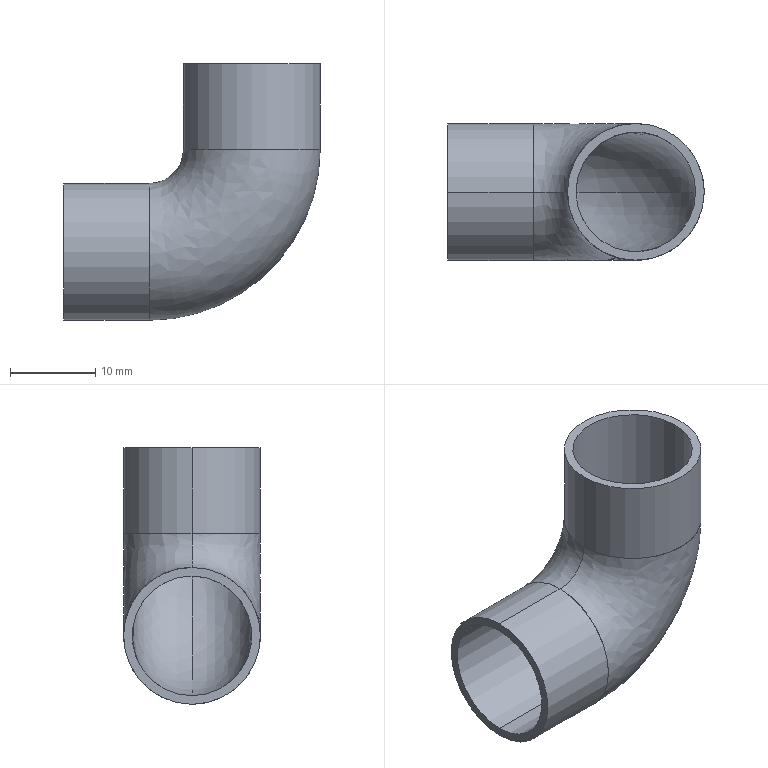Part | STEP file | five-eighths elbow_default_machined_ | 3 solids | 18 faces | box 30 x 16 x 30 mm | volume 1831 mm3 | cylinder 8 | plane 6 | spline 4 | commonest cylinder face diameters 14 x4 16 x4